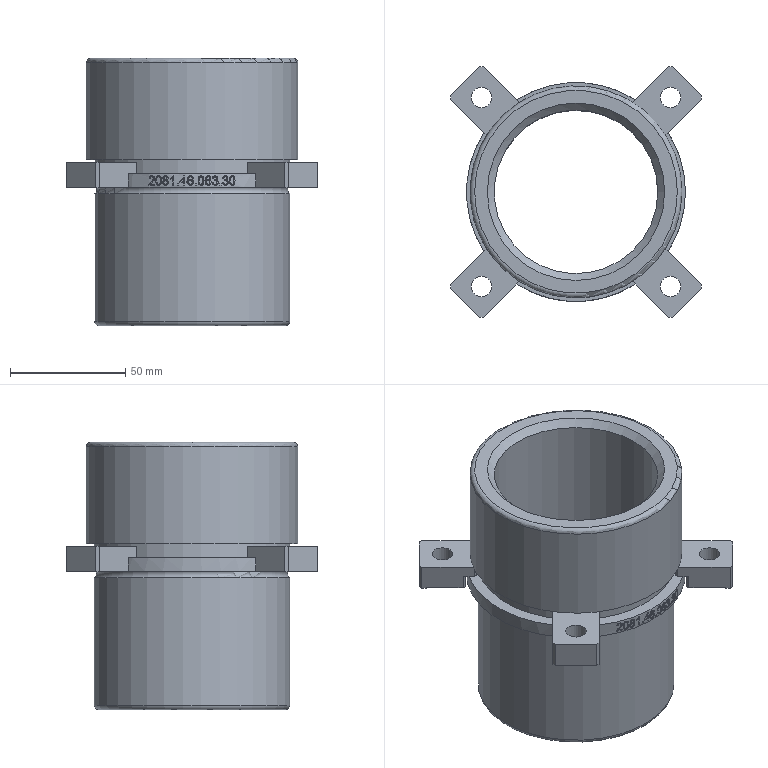Part | NX | features solid 2 | 1 solid | 191 faces | box 108.894 x 108.894 x 116 mm | volume 263259 mm3 | plane 101 | spline 54 | cylinder 31 | torus 3 | cone 2 | commonest cylinder face diameters 94.98 x14 95 x9 9 x4 85 x2 71 x1 92 x1